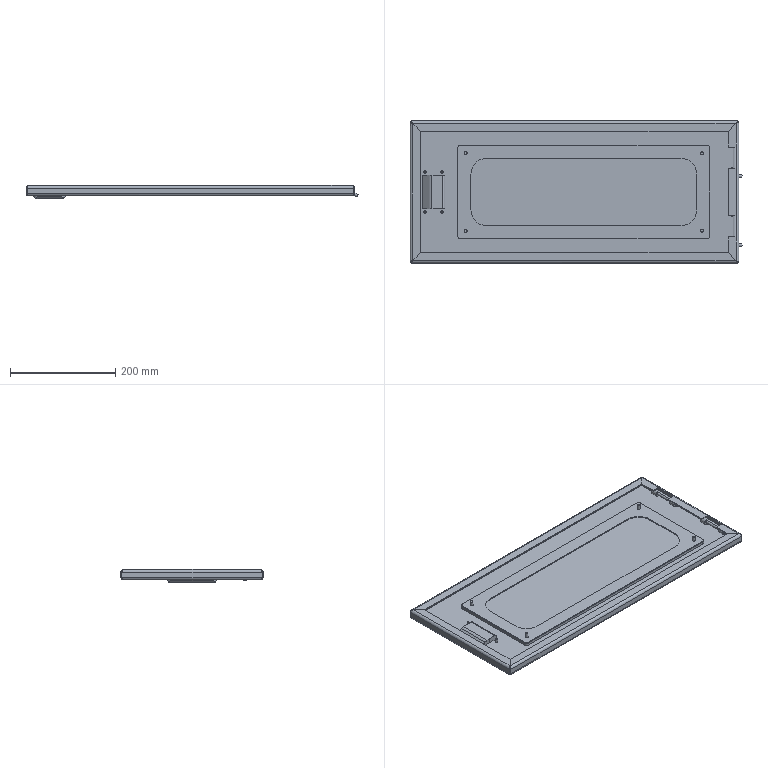Part | SolidWorks | features MirrorCompFeat 1, ReferencePattern 1 | 8 solids | 254 faces | box 632.212 x 271 x 25 mm | volume 870421 mm3 | plane 133 | cylinder 93 | spline 16 | cone 8 | torus 4 | commonest cylinder face diameters 6 x28 5 x24 10 x16 4 x8 60 x8 20 x4